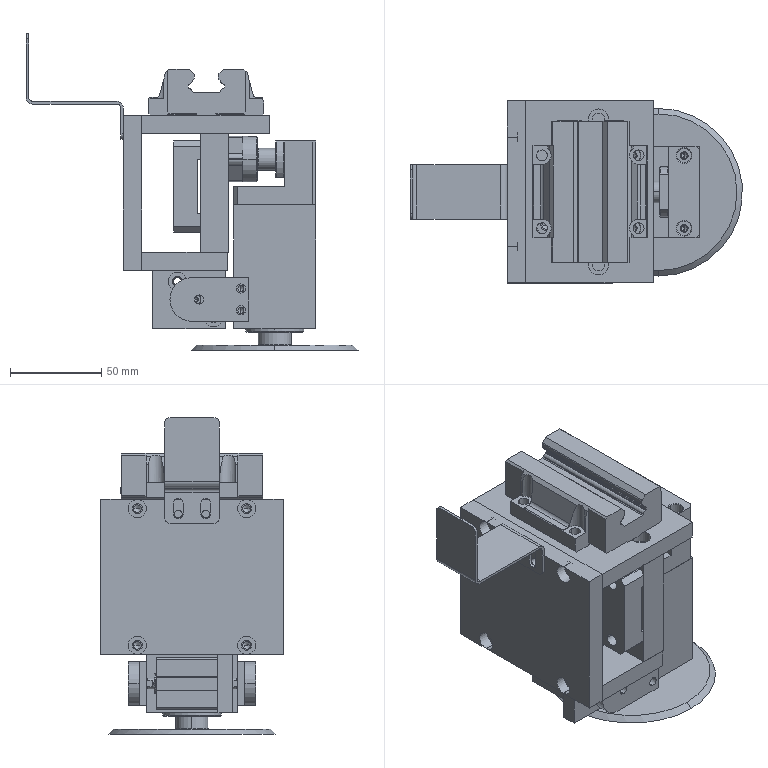Part | SolidWorks | features CompositeCurve 1 | 21 solids | 1135 faces | box 182.5 x 100 x 174 mm | volume 654284 mm3 | plane 521 | cylinder 392 | cone 150 | spline 72 | commonest cylinder face diameters 5 x38 6 x30 1 x24 11 x24 4.2 x22 3.3 x20